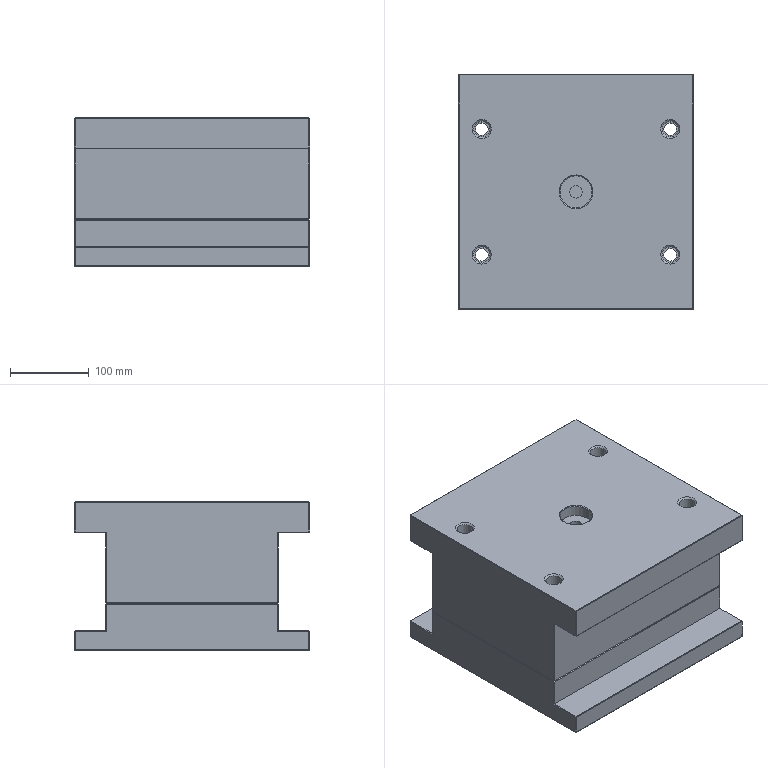Part | 2 solids | 289 faces | box 300 x 300 x 190 mm | volume 13370608 mm3 | plane 221 | spline 24 | cylinder 23 | cone 20 | torus 1 | commonest cylinder face diameters 16 x5 15.98 x4 20 x4 22 x4 34 x2 41 x1